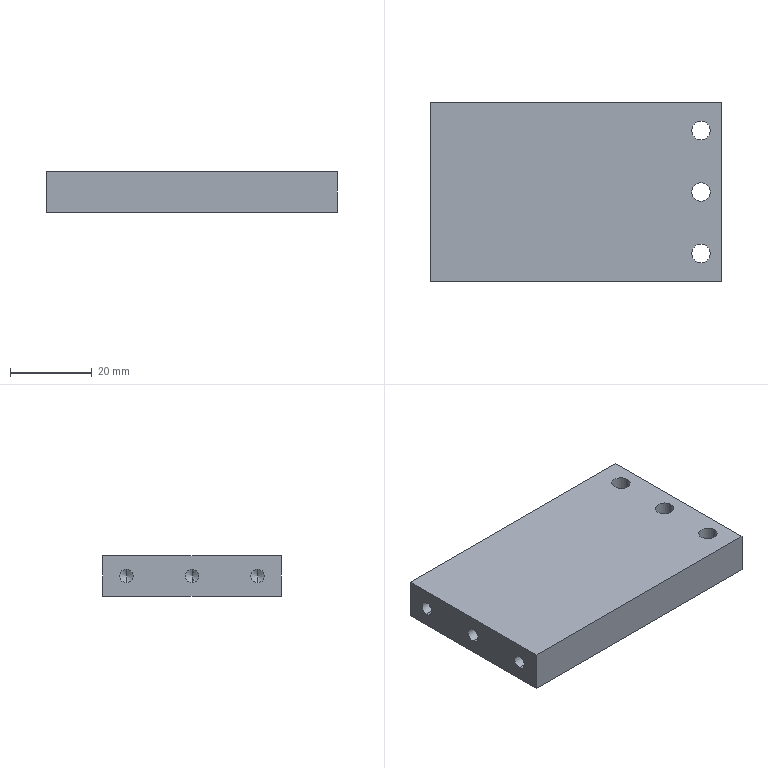Part | SolidWorks | features HoleWzd 2, Extrusion 1 | 1 solid | 33 faces | box 71 x 43.6 x 10 mm | volume 29737 mm3 | cylinder 18 | plane 9 | cone 6 | commonest cylinder face diameters 3.3 x6 4.5 x6 8 x6
STEP:
#1=CARTESIAN_POINT('',(10.1,37.8,-6.65));
#2=VERTEX_POINT('',#1);
#3=CARTESIAN_POINT('',(10.1,37.8,-3.35));
#4=VERTEX_POINT('',#3);
#5=CARTESIAN_POINT('',(10.1,37.8,-5.));
#6=DIRECTION('',(-1.,0.,0.));
#7=DIRECTION('',(0.,0.,1.));
#8=AXIS2_PLACEMENT_3D('',#5,#6,#7);
#9=CIRCLE('',#8,1.65);
#10=EDGE_CURVE('',#2,#4,#9,.T.);
#11=ORIENTED_EDGE('',*,*,#10,.F.);
#12=CARTESIAN_POINT('',(0.,37.8,-6.65));
#13=VERTEX_POINT('',#12);
#14=CARTESIAN_POINT('',(0.,37.8,-6.65));
#15=DIRECTION('',(-1.,0.,0.));
#16=VECTOR('',#15,1000.);
#17=LINE('',#14,#16);
#18=EDGE_CURVE('',#2,#13,#17,.T.);
#19=ORIENTED_EDGE('',*,*,#18,.T.);
#20=CARTESIAN_POINT('',(0.,37.8,-3.35));
#21=VERTEX_POINT('',#20);
#22=CARTESIAN_POINT('',(0.,37.8,-5.));
#23=DIRECTION('',(-1.,0.,0.));
#24=DIRECTION('',(0.,0.,1.));
#25=AXIS2_PLACEMENT_3D('',#22,#23,#24);
#26=CIRCLE('',#25,1.65);
#27=EDGE_CURVE('',#13,#21,#26,.T.);
#28=ORIENTED_EDGE('',*,*,#27,.T.);
#29=CARTESIAN_POINT('',(0.,37.8,-3.35));
#30=DIRECTION('',(-1.,0.,0.));
#31=VECTOR('',#30,1000.);
#32=LINE('',#29,#31);
#33=EDGE_CURVE('',#4,#21,#32,.T.);
#34=ORIENTED_EDGE('',*,*,#33,.F.);
#35=EDGE_LOOP('',(#11,#19,#28,#34));
#36=FACE_OUTER_BOUND('',#35,.T.);
#37=CARTESIAN_POINT('',(0.,37.8,-5.));
#38=DIRECTION('',(-1.,0.,0.));
#39=DIRECTION('',(0.,0.,1.));
#40=AXIS2_PLACEMENT_3D('',#37,#38,#39);
#41=CYLINDRICAL_SURFACE('',#40,1.65);
#42=ADVANCED_FACE('',(#36),#41,.F.);
#43=CARTESIAN_POINT('',(11.091,37.8,-5.));
#44=VERTEX_POINT('',#43);
#45=CARTESIAN_POINT('',(10.1,37.8,-3.35));
#46=DIRECTION('',(-0.515,0.,0.8572));
#47=VECTOR('',#46,1000.);
#48=LINE('',#45,#47);
#49=EDGE_CURVE('',#44,#4,#48,.T.);
#50=ORIENTED_EDGE('',*,*,#49,.F.);
#51=CARTESIAN_POINT('',(10.1,37.8,-6.65));
#52=DIRECTION('',(-0.515,0.,-0.8572));
#53=VECTOR('',#52,1000.);
#54=LINE('',#51,#53);
#55=EDGE_CURVE('',#44,#2,#54,.T.);
#56=ORIENTED_EDGE('',*,*,#55,.T.);
#57=ORIENTED_EDGE('',*,*,#10,.T.);
#58=EDGE_LOOP('',(#50,#56,#57));
#59=FACE_OUTER_BOUND('',#58,.T.);
#60=CARTESIAN_POINT('',(10.1,37.8,-5.));
#61=DIRECTION('',(-1.,0.,0.));
#62=DIRECTION('',(0.,0.,1.));
#63=AXIS2_PLACEMENT_3D('',#60,#61,#62);
#64=CONICAL_SURFACE('',#63,1.65,1.03);
#65=ADVANCED_FACE('',(#59),#64,.F.);
#66=CARTESIAN_POINT('',(10.1,21.8,-6.65));
#67=VERTEX_POINT('',#66);
#68=CARTESIAN_POINT('',(10.1,21.8,-3.35));
#69=VERTEX_POINT('',#68);
#70=CARTESIAN_POINT('',(10.1,21.8,-5.));
#71=DIRECTION('',(-1.,0.,0.));
#72=DIRECTION('',(0.,0.,1.));
#73=AXIS2_PLACEMENT_3D('',#70,#71,#72);
#74=CIRCLE('',#73,1.65);
#75=EDGE_CURVE('',#67,#69,#74,.T.);
#76=ORIENTED_EDGE('',*,*,#75,.F.);
#77=CARTESIAN_POINT('',(0.,21.8,-6.65));
#78=VERTEX_POINT('',#77);
#79=CARTESIAN_POINT('',(0.,21.8,-6.65));
#80=DIRECTION('',(-1.,0.,0.));
#81=VECTOR('',#80,1000.);
#82=LINE('',#79,#81);
#83=EDGE_CURVE('',#67,#78,#82,.T.);
#84=ORIENTED_EDGE('',*,*,#83,.T.);
#85=CARTESIAN_POINT('',(0.,21.8,-3.35));
#86=VERTEX_POINT('',#85);
#87=CARTESIAN_POINT('',(0.,21.8,-5.));
#88=DIRECTION('',(-1.,0.,0.));
#89=DIRECTION('',(0.,0.,1.));
#90=AXIS2_PLACEMENT_3D('',#87,#88,#89);
#91=CIRCLE('',#90,1.65);
#92=EDGE_CURVE('',#78,#86,#91,.T.);
#93=ORIENTED_EDGE('',*,*,#92,.T.);
#94=CARTESIAN_POINT('',(0.,21.8,-3.35));
#95=DIRECTION('',(-1.,0.,0.));
#96=VECTOR('',#95,1000.);
#97=LINE('',#94,#96);
#98=EDGE_CURVE('',#69,#86,#97,.T.);
#99=ORIENTED_EDGE('',*,*,#98,.F.);
#100=EDGE_LOOP('',(#76,#84,#93,#99));
#101=FACE_OUTER_BOUND('',#100,.T.);
#102=CARTESIAN_POINT('',(0.,21.8,-5.));
#103=DIRECTION('',(-1.,0.,0.));
#104=DIRECTION('',(0.,0.,1.));
#105=AXIS2_PLACEMENT_3D('',#102,#103,#104);
#106=CYLINDRICAL_SURFACE('',#105,1.65);
#107=ADVANCED_FACE('',(#101),#106,.F.);
#108=CARTESIAN_POINT('',(11.091,21.8,-5.));
#109=VERTEX_POINT('',#108);
#110=CARTESIAN_POINT('',(10.1,21.8,-3.35));
#111=DIRECTION('',(-0.515,0.,0.8572));
#112=VECTOR('',#111,1000.);
#113=LINE('',#110,#112);
#114=EDGE_CURVE('',#109,#69,#113,.T.);
#115=ORIENTED_EDGE('',*,*,#114,.F.);
#116=CARTESIAN_POINT('',(10.1,21.8,-6.65));
#117=DIRECTION('',(-0.515,0.,-0.8572));
#118=VECTOR('',#117,1000.);
#119=LINE('',#116,#118);
#120=EDGE_CURVE('',#109,#67,#119,.T.);
#121=ORIENTED_EDGE('',*,*,#120,.T.);
#122=ORIENTED_EDGE('',*,*,#75,.T.);
#123=EDGE_LOOP('',(#115,#121,#122));
#124=FACE_OUTER_BOUND('',#123,.T.);
#125=CARTESIAN_POINT('',(10.1,21.8,-5.));
#126=DIRECTION('',(-1.,0.,0.));
#127=DIRECTION('',(0.,0.,1.));
#128=AXIS2_PLACEMENT_3D('',#125,#126,#127);
#129=CONICAL_SURFACE('',#128,1.65,1.03);
#130=ADVANCED_FACE('',(#124),#129,.F.);
#131=CARTESIAN_POINT('',(10.1,5.8,-6.65));
#132=VERTEX_POINT('',#131);
#133=CARTESIAN_POINT('',(10.1,5.8,-3.35));
#134=VERTEX_POINT('',#133);
#135=CARTESIAN_POINT('',(10.1,5.8,-5.));
#136=DIRECTION('',(-1.,0.,0.));
#137=DIRECTION('',(0.,0.,1.));
#138=AXIS2_PLACEMENT_3D('',#135,#136,#137);
#139=CIRCLE('',#138,1.65);
#140=EDGE_CURVE('',#132,#134,#139,.T.);
#141=ORIENTED_EDGE('',*,*,#140,.F.);
#142=CARTESIAN_POINT('',(0.,5.8,-6.65));
#143=VERTEX_POINT('',#142);
#144=CARTESIAN_POINT('',(0.,5.8,-6.65));
#145=DIRECTION('',(-1.,0.,0.));
#146=VECTOR('',#145,1000.);
#147=LINE('',#144,#146);
#148=EDGE_CURVE('',#132,#143,#147,.T.);
#149=ORIENTED_EDGE('',*,*,#148,.T.);
#150=CARTESIAN_POINT('',(0.,5.8,-3.35));
#151=VERTEX_POINT('',#150);
#152=CARTESIAN_POINT('',(0.,5.8,-5.));
#153=DIRECTION('',(-1.,0.,0.));
#154=DIRECTION('',(0.,0.,1.));
#155=AXIS2_PLACEMENT_3D('',#152,#153,#154);
#156=CIRCLE('',#155,1.65);
#157=EDGE_CURVE('',#143,#151,#156,.T.);
#158=ORIENTED_EDGE('',*,*,#157,.T.);
#159=CARTESIAN_POINT('',(0.,5.8,-3.35));
#160=DIRECTION('',(-1.,0.,0.));
#161=VECTOR('',#160,1000.);
#162=LINE('',#159,#161);
#163=EDGE_CURVE('',#134,#151,#162,.T.);
#164=ORIENTED_EDGE('',*,*,#163,.F.);
#165=EDGE_LOOP('',(#141,#149,#158,#164));
#166=FACE_OUTER_BOUND('',#165,.T.);
#167=CARTESIAN_POINT('',(0.,5.8,-5.));
#168=DIRECTION('',(-1.,0.,0.));
#169=DIRECTION('',(0.,0.,1.));
#170=AXIS2_PLACEMENT_3D('',#167,#168,#169);
#171=CYLINDRICAL_SURFACE('',#170,1.65);
#172=ADVANCED_FACE('',(#166),#171,.F.);
#173=CARTESIAN_POINT('',(11.091,5.8,-5.));
#174=VERTEX_POINT('',#173);
#175=CARTESIAN_POINT('',(10.1,5.8,-3.35));
#176=DIRECTION('',(-0.515,0.,0.8572));
#177=VECTOR('',#176,1000.);
#178=LINE('',#175,#177);
#179=EDGE_CURVE('',#174,#134,#178,.T.);
#180=ORIENTED_EDGE('',*,*,#179,.F.);
#181=CARTESIAN_POINT('',(10.1,5.8,-6.65));
#182=DIRECTION('',(-0.515,0.,-0.8572));
#183=VECTOR('',#182,1000.);
#184=LINE('',#181,#183);
#185=EDGE_CURVE('',#174,#132,#184,.T.);
#186=ORIENTED_EDGE('',*,*,#185,.T.);
#187=ORIENTED_EDGE('',*,*,#140,.T.);
#188=EDGE_LOOP('',(#180,#186,#187));
#189=FACE_OUTER_BOUND('',#188,.T.);
#190=CARTESIAN_POINT('',(10.1,5.8,-5.));
#191=DIRECTION('',(-1.,0.,0.));
#192=DIRECTION('',(0.,0.,1.));
#193=AXIS2_PLACEMENT_3D('',#190,#191,#192);
#194=CONICAL_SURFACE('',#193,1.65,1.03);
#195=ADVANCED_FACE('',(#189),#194,.F.);
#196=CARTESIAN_POINT('',(70.,36.8,-5.4));
#197=VERTEX_POINT('',#196);
#198=CARTESIAN_POINT('',(62.,36.8,-5.4));
#199=VERTEX_POINT('',#198);
#200=CARTESIAN_POINT('',(66.,36.8,-5.4));
#201=DIRECTION('',(0.,0.,-1.));
#202=DIRECTION('',(-1.,0.,0.));
#203=AXIS2_PLACEMENT_3D('',#200,#201,#202);
#204=CIRCLE('',#203,4.);
#205=EDGE_CURVE('',#197,#199,#204,.T.);
#206=ORIENTED_EDGE('',*,*,#205,.F.);
#207=CARTESIAN_POINT('',(70.,36.8,-10.));
#208=VERTEX_POINT('',#207);
#209=CARTESIAN_POINT('',(70.,36.8,-10.));
#210=DIRECTION('',(0.,0.,-1.));
#211=VECTOR('',#210,1000.);
#212=LINE('',#209,#211);
#213=EDGE_CURVE('',#197,#208,#212,.T.);
#214=ORIENTED_EDGE('',*,*,#213,.T.);
#215=CARTESIAN_POINT('',(62.,36.8,-10.));
#216=VERTEX_POINT('',#215);
#217=CARTESIAN_POINT('',(66.,36.8,-10.));
#218=DIRECTION('',(0.,0.,-1.));
#219=DIRECTION('',(-1.,0.,0.));
#220=AXIS2_PLACEMENT_3D('',#217,#218,#219);
#221=CIRCLE('',#220,4.);
#222=EDGE_CURVE('',#208,#216,#221,.T.);
#223=ORIENTED_EDGE('',*,*,#222,.T.);
#224=CARTESIAN_POINT('',(62.,36.8,-10.));
#225=DIRECTION('',(0.,0.,-1.));
#226=VECTOR('',#225,1000.);
#227=LINE('',#224,#226);
#228=EDGE_CURVE('',#199,#216,#227,.T.);
#229=ORIENTED_EDGE('',*,*,#228,.F.);
#230=EDGE_LOOP('',(#206,#214,#223,#229));
#231=FACE_OUTER_BOUND('',#230,.T.);
#232=CARTESIAN_POINT('',(66.,36.8,-10.));
#233=DIRECTION('',(0.,0.,-1.));
#234=DIRECTION('',(-1.,0.,0.));
#235=AXIS2_PLACEMENT_3D('',#232,#233,#234);
#236=CYLINDRICAL_SURFACE('',#235,4.);
#237=ADVANCED_FACE('',(#231),#236,.F.);
#238=CARTESIAN_POINT('',(68.25,36.8,0.));
#239=VERTEX_POINT('',#238);
#240=CARTESIAN_POINT('',(63.75,36.8,0.));
#241=VERTEX_POINT('',#240);
#242=CARTESIAN_POINT('',(66.,36.8,0.));
#243=DIRECTION('',(0.,0.,-1.));
#244=DIRECTION('',(-1.,0.,0.));
#245=AXIS2_PLACEMENT_3D('',#242,#243,#244);
#246=CIRCLE('',#245,2.25);
#247=EDGE_CURVE('',#239,#241,#246,.T.);
#248=ORIENTED_EDGE('',*,*,#247,.F.);
#249=CARTESIAN_POINT('',(68.25,36.8,-5.4));
#250=VERTEX_POINT('',#249);
#251=CARTESIAN_POINT('',(68.25,36.8,-10.));
#252=DIRECTION('',(0.,0.,-1.));
#253=VECTOR('',#252,1000.);
#254=LINE('',#251,#253);
#255=EDGE_CURVE('',#239,#250,#254,.T.);
#256=ORIENTED_EDGE('',*,*,#255,.T.);
#257=CARTESIAN_POINT('',(63.75,36.8,-5.4));
#258=VERTEX_POINT('',#257);
#259=CARTESIAN_POINT('',(66.,36.8,-5.4));
#260=DIRECTION('',(0.,0.,-1.));
#261=DIRECTION('',(-1.,0.,0.));
#262=AXIS2_PLACEMENT_3D('',#259,#260,#261);
#263=CIRCLE('',#262,2.25);
#264=EDGE_CURVE('',#250,#258,#263,.T.);
#265=ORIENTED_EDGE('',*,*,#264,.T.);
#266=CARTESIAN_POINT('',(63.75,36.8,-10.));
#267=DIRECTION('',(0.,0.,-1.));
#268=VECTOR('',#267,1000.);
#269=LINE('',#266,#268);
#270=EDGE_CURVE('',#241,#258,#269,.T.);
#271=ORIENTED_EDGE('',*,*,#270,.F.);
#272=EDGE_LOOP('',(#248,#256,#265,#271));
#273=FACE_OUTER_BOUND('',#272,.T.);
#274=CARTESIAN_POINT('',(66.,36.8,-10.));
#275=DIRECTION('',(0.,0.,-1.));
#276=DIRECTION('',(-1.,0.,0.));
#277=AXIS2_PLACEMENT_3D('',#274,#275,#276);
#278=CYLINDRICAL_SURFACE('',#277,2.25);
#279=ADVANCED_FACE('',(#273),#278,.F.);
#280=CARTESIAN_POINT('',(70.,21.783,-5.4));
#281=VERTEX_POINT('',#280);
#282=CARTESIAN_POINT('',(62.,21.783,-5.4));
#283=VERTEX_POINT('',#282);
#284=CARTESIAN_POINT('',(66.,21.783,-5.4));
#285=DIRECTION('',(0.,0.,-1.));
#286=DIRECTION('',(-1.,0.,0.));
#287=AXIS2_PLACEMENT_3D('',#284,#285,#286);
#288=CIRCLE('',#287,4.);
#289=EDGE_CURVE('',#281,#283,#288,.T.);
#290=ORIENTED_EDGE('',*,*,#289,.F.);
#291=CARTESIAN_POINT('',(70.,21.783,-10.));
#292=VERTEX_POINT('',#291);
#293=CARTESIAN_POINT('',(70.,21.783,-10.));
#294=DIRECTION('',(0.,0.,-1.));
#295=VECTOR('',#294,1000.);
#296=LINE('',#293,#295);
#297=EDGE_CURVE('',#281,#292,#296,.T.);
#298=ORIENTED_EDGE('',*,*,#297,.T.);
#299=CARTESIAN_POINT('',(62.,21.783,-10.));
#300=VERTEX_POINT('',#299);
#301=CARTESIAN_POINT('',(66.,21.783,-10.));
#302=DIRECTION('',(0.,0.,-1.));
#303=DIRECTION('',(-1.,0.,0.));
#304=AXIS2_PLACEMENT_3D('',#301,#302,#303);
#305=CIRCLE('',#304,4.);
#306=EDGE_CURVE('',#292,#300,#305,.T.);
#307=ORIENTED_EDGE('',*,*,#306,.T.);
#308=CARTESIAN_POINT('',(62.,21.783,-10.));
#309=DIRECTION('',(0.,0.,-1.));
#310=VECTOR('',#309,1000.);
#311=LINE('',#308,#310);
#312=EDGE_CURVE('',#283,#300,#311,.T.);
#313=ORIENTED_EDGE('',*,*,#312,.F.);
#314=EDGE_LOOP('',(#290,#298,#307,#313));
#315=FACE_OUTER_BOUND('',#314,.T.);
#316=CARTESIAN_POINT('',(66.,21.783,-10.));
#317=DIRECTION('',(0.,0.,-1.));
#318=DIRECTION('',(-1.,0.,0.));
#319=AXIS2_PLACEMENT_3D('',#316,#317,#318);
#320=CYLINDRICAL_SURFACE('',#319,4.);
#321=ADVANCED_FACE('',(#315),#320,.F.);
#322=CARTESIAN_POINT('',(68.25,21.783,0.));
#323=VERTEX_POINT('',#322);
#324=CARTESIAN_POINT('',(63.75,21.783,0.));
#325=VERTEX_POINT('',#324);
#326=CARTESIAN_POINT('',(66.,21.783,0.));
#327=DIRECTION('',(0.,0.,-1.));
#328=DIRECTION('',(-1.,0.,0.));
#329=AXIS2_PLACEMENT_3D('',#326,#327,#328);
#330=CIRCLE('',#329,2.25);
#331=EDGE_CURVE('',#323,#325,#330,.T.);
#332=ORIENTED_EDGE('',*,*,#331,.F.);
#333=CARTESIAN_POINT('',(68.25,21.783,-5.4));
#334=VERTEX_POINT('',#333);
#335=CARTESIAN_POINT('',(68.25,21.783,-10.));
#336=DIRECTION('',(0.,0.,-1.));
#337=VECTOR('',#336,1000.);
#338=LINE('',#335,#337);
#339=EDGE_CURVE('',#323,#334,#338,.T.);
#340=ORIENTED_EDGE('',*,*,#339,.T.);
#341=CARTESIAN_POINT('',(63.75,21.783,-5.4));
#342=VERTEX_POINT('',#341);
#343=CARTESIAN_POINT('',(66.,21.783,-5.4));
#344=DIRECTION('',(0.,0.,-1.));
#345=DIRECTION('',(-1.,0.,0.));
#346=AXIS2_PLACEMENT_3D('',#343,#344,#345);
#347=CIRCLE('',#346,2.25);
#348=EDGE_CURVE('',#334,#342,#347,.T.);
#349=ORIENTED_EDGE('',*,*,#348,.T.);
#350=CARTESIAN_POINT('',(63.75,21.783,-10.));
#351=DIRECTION('',(0.,0.,-1.));
#352=VECTOR('',#351,1000.);
#353=LINE('',#350,#352);
#354=EDGE_CURVE('',#325,#342,#353,.T.);
#355=ORIENTED_EDGE('',*,*,#354,.F.);
#356=EDGE_LOOP('',(#332,#340,#349,#355));
#357=FACE_OUTER_BOUND('',#356,.T.);
#358=CARTESIAN_POINT('',(66.,21.783,-10.));
#359=DIRECTION('',(0.,0.,-1.));
#360=DIRECTION('',(-1.,0.,0.));
#361=AXIS2_PLACEMENT_3D('',#358,#359,#360);
#362=CYLINDRICAL_SURFACE('',#361,2.25);
#363=ADVANCED_FACE('',(#357),#362,.F.);
#364=CARTESIAN_POINT('',(70.,6.8,-5.4));
#365=VERTEX_POINT('',#364);
#366=CARTESIAN_POINT('',(62.,6.8,-5.4));
#367=VERTEX_POINT('',#366);
#368=CARTESIAN_POINT('',(66.,6.8,-5.4));
#369=DIRECTION('',(0.,0.,-1.));
#370=DIRECTION('',(-1.,0.,0.));
#371=AXIS2_PLACEMENT_3D('',#368,#369,#370);
#372=CIRCLE('',#371,4.);
#373=EDGE_CURVE('',#365,#367,#372,.T.);
#374=ORIENTED_EDGE('',*,*,#373,.F.);
#375=CARTESIAN_POINT('',(70.,6.8,-10.));
#376=VERTEX_POINT('',#375);
#377=CARTESIAN_POINT('',(70.,6.8,-10.));
#378=DIRECTION('',(0.,0.,-1.));
#379=VECTOR('',#378,1000.);
#380=LINE('',#377,#379);
#381=EDGE_CURVE('',#365,#376,#380,.T.);
#382=ORIENTED_EDGE('',*,*,#381,.T.);
#383=CARTESIAN_POINT('',(62.,6.8,-10.));
#384=VERTEX_POINT('',#383);
#385=CARTESIAN_POINT('',(66.,6.8,-10.));
#386=DIRECTION('',(0.,0.,-1.));
#387=DIRECTION('',(-1.,0.,0.));
#388=AXIS2_PLACEMENT_3D('',#385,#386,#387);
#389=CIRCLE('',#388,4.);
#390=EDGE_CURVE('',#376,#384,#389,.T.);
#391=ORIENTED_EDGE('',*,*,#390,.T.);
#392=CARTESIAN_POINT('',(62.,6.8,-10.));
#393=DIRECTION('',(0.,0.,-1.));
#394=VECTOR('',#393,1000.);
#395=LINE('',#392,#394);
#396=EDGE_CURVE('',#367,#384,#395,.T.);
#397=ORIENTED_EDGE('',*,*,#396,.F.);
#398=EDGE_LOOP('',(#374,#382,#391,#397));
#399=FACE_OUTER_BOUND('',#398,.T.);
#400=CARTESIAN_POINT('',(66.,6.8,-10.));
#401=DIRECTION('',(0.,0.,-1.));
#402=DIRECTION('',(-1.,0.,0.));
#403=AXIS2_PLACEMENT_3D('',#400,#401,#402);
#404=CYLINDRICAL_SURFACE('',#403,4.);
#405=ADVANCED_FACE('',(#399),#404,.F.);
#406=CARTESIAN_POINT('',(68.25,6.8,0.));
#407=VERTEX_POINT('',#406);
#408=CARTESIAN_POINT('',(63.75,6.8,0.));
#409=VERTEX_POINT('',#408);
#410=CARTESIAN_POINT('',(66.,6.8,0.));
#411=DIRECTION('',(0.,0.,-1.));
#412=DIRECTION('',(-1.,0.,0.));
#413=AXIS2_PLACEMENT_3D('',#410,#411,#412);
#414=CIRCLE('',#413,2.25);
#415=EDGE_CURVE('',#407,#409,#414,.T.);
#416=ORIENTED_EDGE('',*,*,#415,.F.);
#417=CARTESIAN_POINT('',(68.25,6.8,-5.4));
#418=VERTEX_POINT('',#417);
#419=CARTESIAN_POINT('',(68.25,6.8,-10.));
#420=DIRECTION('',(0.,0.,-1.));
#421=VECTOR('',#420,1000.);
#422=LINE('',#419,#421);
#423=EDGE_CURVE('',#407,#418,#422,.T.);
#424=ORIENTED_EDGE('',*,*,#423,.T.);
#425=CARTESIAN_POINT('',(63.75,6.8,-5.4));
#426=VERTEX_POINT('',#425);
#427=CARTESIAN_POINT('',(66.,6.8,-5.4));
#428=DIRECTION('',(0.,0.,-1.));
#429=DIRECTION('',(-1.,0.,0.));
#430=AXIS2_PLACEMENT_3D('',#427,#428,#429);
#431=CIRCLE('',#430,2.25);
#432=EDGE_CURVE('',#418,#426,#431,.T.);
#433=ORIENTED_EDGE('',*,*,#432,.T.);
#434=CARTESIAN_POINT('',(63.75,6.8,-10.));
#435=DIRECTION('',(0.,0.,-1.));
#436=VECTOR('',#435,1000.);
#437=LINE('',#434,#436);
#438=EDGE_CURVE('',#409,#426,#437,.T.);
#439=ORIENTED_EDGE('',*,*,#438,.F.);
#440=EDGE_LOOP('',(#416,#424,#433,#439));
#441=FACE_OUTER_BOUND('',#440,.T.);
#442=CARTESIAN_POINT('',(66.,6.8,-10.));
#443=DIRECTION('',(0.,0.,-1.));
#444=DIRECTION('',(-1.,0.,0.));
#445=AXIS2_PLACEMENT_3D('',#442,#443,#444);
#446=CYLINDRICAL_SURFACE('',#445,2.25);
#447=ADVANCED_FACE('',(#441),#446,.F.);
#448=CARTESIAN_POINT('',(0.,37.8,-5.));
#449=DIRECTION('',(-1.,0.,0.));
#450=DIRECTION('',(0.,0.,1.));
#451=AXIS2_PLACEMENT_3D('',#448,#449,#450);
#452=CIRCLE('',#451,1.65);
#453=EDGE_CURVE('',#21,#13,#452,.T.);
#454=ORIENTED_EDGE('',*,*,#453,.F.);
#455=ORIENTED_EDGE('',*,*,#27,.F.);
#456=EDGE_LOOP('',(#454,#455));
#457=FACE_BOUND('',#456,.T.);
#458=CARTESIAN_POINT('',(0.,21.8,-5.));
#459=DIRECTION('',(-1.,0.,0.));
#460=DIRECTION('',(0.,0.,1.));
#461=AXIS2_PLACEMENT_3D('',#458,#459,#460);
#462=CIRCLE('',#461,1.65);
#463=EDGE_CURVE('',#86,#78,#462,.T.);
#464=ORIENTED_EDGE('',*,*,#463,.F.);
#465=ORIENTED_EDGE('',*,*,#92,.F.);
#466=EDGE_LOOP('',(#464,#465));
#467=FACE_BOUND('',#466,.T.);
#468=CARTESIAN_POINT('',(0.,5.8,-5.));
#469=DIRECTION('',(-1.,0.,0.));
#470=DIRECTION('',(0.,0.,1.));
#471=AXIS2_PLACEMENT_3D('',#468,#469,#470);
#472=CIRCLE('',#471,1.65);
#473=EDGE_CURVE('',#151,#143,#472,.T.);
#474=ORIENTED_EDGE('',*,*,#473,.F.);
#475=ORIENTED_EDGE('',*,*,#157,.F.);
#476=EDGE_LOOP('',(#474,#475));
#477=FACE_BOUND('',#476,.T.);
#478=CARTESIAN_POINT('',(0.,0.,-10.));
#479=VERTEX_POINT('',#478);
#480=CARTESIAN_POINT('',(0.,0.,0.));
#481=VERTEX_POINT('',#480);
#482=CARTESIAN_POINT('',(0.,0.,0.));
#483=DIRECTION('',(0.,0.,1.));
#484=VECTOR('',#483,1000.);
#485=LINE('',#482,#484);
#486=EDGE_CURVE('',#479,#481,#485,.T.);
#487=ORIENTED_EDGE('',*,*,#486,.T.);
#488=CARTESIAN_POINT('',(0.,43.6,0.));
#489=VERTEX_POINT('',#488);
#490=CARTESIAN_POINT('',(0.,43.6,0.));
#491=DIRECTION('',(0.,-1.,0.));
#492=VECTOR('',#491,1000.);
#493=LINE('',#490,#492);
#494=EDGE_CURVE('',#489,#481,#493,.T.);
#495=ORIENTED_EDGE('',*,*,#494,.F.);
#496=CARTESIAN_POINT('',(0.,43.6,-10.));
#497=VERTEX_POINT('',#496);
#498=CARTESIAN_POINT('',(0.,43.6,0.));
#499=DIRECTION('',(0.,0.,1.));
#500=VECTOR('',#499,1000.);
#501=LINE('',#498,#500);
#502=EDGE_CURVE('',#497,#489,#501,.T.);
#503=ORIENTED_EDGE('',*,*,#502,.F.);
#504=CARTESIAN_POINT('',(0.,43.6,-10.));
#505=DIRECTION('',(0.,-1.,0.));
#506=VECTOR('',#505,1000.);
#507=LINE('',#504,#506);
#508=EDGE_CURVE('',#497,#479,#507,.T.);
#509=ORIENTED_EDGE('',*,*,#508,.T.);
#510=EDGE_LOOP('',(#487,#495,#503,#509));
#511=FACE_OUTER_BOUND('',#510,.T.);
#512=CARTESIAN_POINT('',(0.,43.6,0.));
#513=DIRECTION('',(1.,0.,0.));
#514=DIRECTION('',(0.,0.,-1.));
#515=AXIS2_PLACEMENT_3D('',#512,#513,#514);
#516=PLANE('',#515);
#517=ADVANCED_FACE('',(#457,#467,#477,#511),#516,.F.);
#518=CARTESIAN_POINT('',(66.,36.8,0.));
#519=DIRECTION('',(0.,0.,-1.));
#520=DIRECTION('',(-1.,0.,0.));
#521=AXIS2_PLACEMENT_3D('',#518,#519,#520);
#522=CIRCLE('',#521,2.25);
#523=EDGE_CURVE('',#241,#239,#522,.T.);
#524=ORIENTED_EDGE('',*,*,#523,.T.);
#525=ORIENTED_EDGE('',*,*,#247,.T.);
#526=EDGE_LOOP('',(#524,#525));
#527=FACE_BOUND('',#526,.T.);
#528=CARTESIAN_POINT('',(66.,21.783,0.));
#529=DIRECTION('',(0.,0.,-1.));
#530=DIRECTION('',(-1.,0.,0.));
#531=AXIS2_PLACEMENT_3D('',#528,#529,#530);
#532=CIRCLE('',#531,2.25);
#533=EDGE_CURVE('',#325,#323,#532,.T.);
#534=ORIENTED_EDGE('',*,*,#533,.T.);
#535=ORIENTED_EDGE('',*,*,#331,.T.);
#536=EDGE_LOOP('',(#534,#535));
#537=FACE_BOUND('',#536,.T.);
#538=CARTESIAN_POINT('',(66.,6.8,0.));
#539=DIRECTION('',(0.,0.,-1.));
#540=DIRECTION('',(-1.,0.,0.));
#541=AXIS2_PLACEMENT_3D('',#538,#539,#540);
#542=CIRCLE('',#541,2.25);
#543=EDGE_CURVE('',#409,#407,#542,.T.);
#544=ORIENTED_EDGE('',*,*,#543,.T.);
#545=ORIENTED_EDGE('',*,*,#415,.T.);
#546=EDGE_LOOP('',(#544,#545));
#547=FACE_BOUND('',#546,.T.);
#548=CARTESIAN_POINT('',(71.,0.,0.));
#549=VERTEX_POINT('',#548);
#550=CARTESIAN_POINT('',(0.,0.,0.));
#551=DIRECTION('',(1.,0.,0.));
#552=VECTOR('',#551,1000.);
#553=LINE('',#550,#552);
#554=EDGE_CURVE('',#481,#549,#553,.T.);
#555=ORIENTED_EDGE('',*,*,#554,.T.);
#556=CARTESIAN_POINT('',(71.,43.6,0.));
#557=VERTEX_POINT('',#556);
#558=CARTESIAN_POINT('',(71.,43.6,0.));
#559=DIRECTION('',(0.,-1.,0.));
#560=VECTOR('',#559,1000.);
#561=LINE('',#558,#560);
#562=EDGE_CURVE('',#557,#549,#561,.T.);
#563=ORIENTED_EDGE('',*,*,#562,.F.);
#564=CARTESIAN_POINT('',(0.,43.6,0.));
#565=DIRECTION('',(1.,0.,0.));
#566=VECTOR('',#565,1000.);
#567=LINE('',#564,#566);
#568=EDGE_CURVE('',#489,#557,#567,.T.);
#569=ORIENTED_EDGE('',*,*,#568,.F.);
#570=ORIENTED_EDGE('',*,*,#494,.T.);
#571=EDGE_LOOP('',(#555,#563,#569,#570));
#572=FACE_OUTER_BOUND('',#571,.T.);
#573=CARTESIAN_POINT('',(0.,43.6,0.));
#574=DIRECTION('',(0.,0.,-1.));
#575=DIRECTION('',(-1.,0.,0.));
#576=AXIS2_PLACEMENT_3D('',#573,#574,#575);
#577=PLANE('',#576);
#578=ADVANCED_FACE('',(#527,#537,#547,#572),#577,.F.);
#579=CARTESIAN_POINT('',(71.,0.,-10.));
#580=VERTEX_POINT('',#579);
#581=CARTESIAN_POINT('',(71.,0.,0.));
#582=DIRECTION('',(0.,0.,-1.));
#583=VECTOR('',#582,1000.);
#584=LINE('',#581,#583);
#585=EDGE_CURVE('',#549,#580,#584,.T.);
#586=ORIENTED_EDGE('',*,*,#585,.T.);
#587=CARTESIAN_POINT('',(71.,43.6,-10.));
#588=VERTEX_POINT('',#587);
#589=CARTESIAN_POINT('',(71.,43.6,-10.));
#590=DIRECTION('',(0.,-1.,0.));
#591=VECTOR('',#590,1000.);
#592=LINE('',#589,#591);
#593=EDGE_CURVE('',#588,#580,#592,.T.);
#594=ORIENTED_EDGE('',*,*,#593,.F.);
#595=CARTESIAN_POINT('',(71.,43.6,0.));
#596=DIRECTION('',(0.,0.,-1.));
#597=VECTOR('',#596,1000.);
#598=LINE('',#595,#597);
#599=EDGE_CURVE('',#557,#588,#598,.T.);
#600=ORIENTED_EDGE('',*,*,#599,.F.);
#601=ORIENTED_EDGE('',*,*,#562,.T.);
#602=EDGE_LOOP('',(#586,#594,#600,#601));
#603=FACE_OUTER_BOUND('',#602,.T.);
#604=CARTESIAN_POINT('',(71.,43.6,0.));
#605=DIRECTION('',(-1.,0.,0.));
#606=DIRECTION('',(0.,0.,1.));
#607=AXIS2_PLACEMENT_3D('',#604,#605,#606);
#608=PLANE('',#607);
#609=ADVANCED_FACE('',(#603),#608,.F.);
#610=CARTESIAN_POINT('',(66.,36.8,-10.));
#611=DIRECTION('',(0.,0.,-1.));
#612=DIRECTION('',(-1.,0.,0.));
#613=AXIS2_PLACEMENT_3D('',#610,#611,#612);
#614=CIRCLE('',#613,4.);
#615=EDGE_CURVE('',#216,#208,#614,.T.);
#616=ORIENTED_EDGE('',*,*,#615,.F.);
#617=ORIENTED_EDGE('',*,*,#222,.F.);
#618=EDGE_LOOP('',(#616,#617));
#619=FACE_BOUND('',#618,.T.);
#620=CARTESIAN_POINT('',(66.,21.783,-10.));
#621=DIRECTION('',(0.,0.,-1.));
#622=DIRECTION('',(-1.,0.,0.));
#623=AXIS2_PLACEMENT_3D('',#620,#621,#622);
#624=CIRCLE('',#623,4.);
#625=EDGE_CURVE('',#300,#292,#624,.T.);
#626=ORIENTED_EDGE('',*,*,#625,.F.);
#627=ORIENTED_EDGE('',*,*,#306,.F.);
#628=EDGE_LOOP('',(#626,#627));
#629=FACE_BOUND('',#628,.T.);
#630=CARTESIAN_POINT('',(66.,6.8,-10.));
#631=DIRECTION('',(0.,0.,-1.));
#632=DIRECTION('',(-1.,0.,0.));
#633=AXIS2_PLACEMENT_3D('',#630,#631,#632);
#634=CIRCLE('',#633,4.);
#635=EDGE_CURVE('',#384,#376,#634,.T.);
#636=ORIENTED_EDGE('',*,*,#635,.F.);
#637=ORIENTED_EDGE('',*,*,#390,.F.);
#638=EDGE_LOOP('',(#636,#637));
#639=FACE_BOUND('',#638,.T.);
#640=CARTESIAN_POINT('',(0.,0.,-10.));
#641=DIRECTION('',(-1.,0.,0.));
#642=VECTOR('',#641,1000.);
#643=LINE('',#640,#642);
#644=EDGE_CURVE('',#580,#479,#643,.T.);
#645=ORIENTED_EDGE('',*,*,#644,.T.);
#646=ORIENTED_EDGE('',*,*,#508,.F.);
#647=CARTESIAN_POINT('',(0.,43.6,-10.));
#648=DIRECTION('',(-1.,0.,0.));
#649=VECTOR('',#648,1000.);
#650=LINE('',#647,#649);
#651=EDGE_CURVE('',#588,#497,#650,.T.);
#652=ORIENTED_EDGE('',*,*,#651,.F.);
#653=ORIENTED_EDGE('',*,*,#593,.T.);
#654=EDGE_LOOP('',(#645,#646,#652,#653));
#655=FACE_OUTER_BOUND('',#654,.T.);
#656=CARTESIAN_POINT('',(0.,43.6,-10.));
#657=DIRECTION('',(0.,0.,1.));
#658=DIRECTION('',(1.,0.,0.));
#659=AXIS2_PLACEMENT_3D('',#656,#657,#658);
#660=PLANE('',#659);
#661=ADVANCED_FACE('',(#619,#629,#639,#655),#660,.F.);
#662=ORIENTED_EDGE('',*,*,#502,.T.);
#663=ORIENTED_EDGE('',*,*,#568,.T.);
#664=ORIENTED_EDGE('',*,*,#599,.T.);
#665=ORIENTED_EDGE('',*,*,#651,.T.);
#666=EDGE_LOOP('',(#662,#663,#664,#665));
#667=FACE_OUTER_BOUND('',#666,.T.);
#668=CARTESIAN_POINT('',(0.,43.6,0.));
#669=DIRECTION('',(0.,-1.,0.));
#670=DIRECTION('',(0.,0.,-1.));
#671=AXIS2_PLACEMENT_3D('',#668,#669,#670);
#672=PLANE('',#671);
#673=ADVANCED_FACE('',(#667),#672,.F.);
#674=ORIENTED_EDGE('',*,*,#486,.F.);
#675=ORIENTED_EDGE('',*,*,#644,.F.);
#676=ORIENTED_EDGE('',*,*,#585,.F.);
#677=ORIENTED_EDGE('',*,*,#554,.F.);
#678=EDGE_LOOP('',(#674,#675,#676,#677));
#679=FACE_OUTER_BOUND('',#678,.T.);
#680=CARTESIAN_POINT('',(0.,0.,0.));
#681=DIRECTION('',(0.,-1.,0.));
#682=DIRECTION('',(0.,0.,-1.));
#683=AXIS2_PLACEMENT_3D('',#680,#681,#682);
#684=PLANE('',#683);
#685=ADVANCED_FACE('',(#679),#684,.T.);
#686=ORIENTED_EDGE('',*,*,#423,.F.);
#687=ORIENTED_EDGE('',*,*,#543,.F.);
#688=ORIENTED_EDGE('',*,*,#438,.T.);
#689=CARTESIAN_POINT('',(66.,6.8,-5.4));
#690=DIRECTION('',(0.,0.,-1.));
#691=DIRECTION('',(-1.,0.,0.));
#692=AXIS2_PLACEMENT_3D('',#689,#690,#691);
#693=CIRCLE('',#692,2.25);
#694=EDGE_CURVE('',#426,#418,#693,.T.);
#695=ORIENTED_EDGE('',*,*,#694,.T.);
#696=EDGE_LOOP('',(#686,#687,#688,#695));
#697=FACE_OUTER_BOUND('',#696,.T.);
#698=CARTESIAN_POINT('',(66.,6.8,-10.));
#699=DIRECTION('',(0.,0.,-1.));
#700=DIRECTION('',(-1.,0.,0.));
#701=AXIS2_PLACEMENT_3D('',#698,#699,#700);
#702=CYLINDRICAL_SURFACE('',#701,2.25);
#703=ADVANCED_FACE('',(#697),#702,.F.);
#704=ORIENTED_EDGE('',*,*,#694,.F.);
#705=ORIENTED_EDGE('',*,*,#432,.F.);
#706=EDGE_LOOP('',(#704,#705));
#707=FACE_BOUND('',#706,.T.);
#708=CARTESIAN_POINT('',(66.,6.8,-5.4));
#709=DIRECTION('',(0.,0.,-1.));
#710=DIRECTION('',(-1.,0.,0.));
#711=AXIS2_PLACEMENT_3D('',#708,#709,#710);
#712=CIRCLE('',#711,4.);
#713=EDGE_CURVE('',#367,#365,#712,.T.);
#714=ORIENTED_EDGE('',*,*,#713,.T.);
#715=ORIENTED_EDGE('',*,*,#373,.T.);
#716=EDGE_LOOP('',(#714,#715));
#717=FACE_OUTER_BOUND('',#716,.T.);
#718=CARTESIAN_POINT('',(68.25,6.8,-5.4));
#719=DIRECTION('',(0.,0.,1.));
#720=DIRECTION('',(1.,0.,0.));
#721=AXIS2_PLACEMENT_3D('',#718,#719,#720);
#722=PLANE('',#721);
#723=ADVANCED_FACE('',(#707,#717),#722,.F.);
#724=ORIENTED_EDGE('',*,*,#381,.F.);
#725=ORIENTED_EDGE('',*,*,#713,.F.);
#726=ORIENTED_EDGE('',*,*,#396,.T.);
#727=ORIENTED_EDGE('',*,*,#635,.T.);
#728=EDGE_LOOP('',(#724,#725,#726,#727));
#729=FACE_OUTER_BOUND('',#728,.T.);
#730=CARTESIAN_POINT('',(66.,6.8,-10.));
#731=DIRECTION('',(0.,0.,-1.));
#732=DIRECTION('',(-1.,0.,0.));
#733=AXIS2_PLACEMENT_3D('',#730,#731,#732);
#734=CYLINDRICAL_SURFACE('',#733,4.);
#735=ADVANCED_FACE('',(#729),#734,.F.);
#736=ORIENTED_EDGE('',*,*,#339,.F.);
#737=ORIENTED_EDGE('',*,*,#533,.F.);
#738=ORIENTED_EDGE('',*,*,#354,.T.);
#739=CARTESIAN_POINT('',(66.,21.783,-5.4));
#740=DIRECTION('',(0.,0.,-1.));
#741=DIRECTION('',(-1.,0.,0.));
#742=AXIS2_PLACEMENT_3D('',#739,#740,#741);
#743=CIRCLE('',#742,2.25);
#744=EDGE_CURVE('',#342,#334,#743,.T.);
#745=ORIENTED_EDGE('',*,*,#744,.T.);
#746=EDGE_LOOP('',(#736,#737,#738,#745));
#747=FACE_OUTER_BOUND('',#746,.T.);
#748=CARTESIAN_POINT('',(66.,21.783,-10.));
#749=DIRECTION('',(0.,0.,-1.));
#750=DIRECTION('',(-1.,0.,0.));
#751=AXIS2_PLACEMENT_3D('',#748,#749,#750);
#752=CYLINDRICAL_SURFACE('',#751,2.25);
#753=ADVANCED_FACE('',(#747),#752,.F.);
#754=ORIENTED_EDGE('',*,*,#744,.F.);
#755=ORIENTED_EDGE('',*,*,#348,.F.);
#756=EDGE_LOOP('',(#754,#755));
#757=FACE_BOUND('',#756,.T.);
#758=CARTESIAN_POINT('',(66.,21.783,-5.4));
#759=DIRECTION('',(0.,0.,-1.));
#760=DIRECTION('',(-1.,0.,0.));
#761=AXIS2_PLACEMENT_3D('',#758,#759,#760);
#762=CIRCLE('',#761,4.);
#763=EDGE_CURVE('',#283,#281,#762,.T.);
#764=ORIENTED_EDGE('',*,*,#763,.T.);
#765=ORIENTED_EDGE('',*,*,#289,.T.);
#766=EDGE_LOOP('',(#764,#765));
#767=FACE_OUTER_BOUND('',#766,.T.);
#768=CARTESIAN_POINT('',(68.25,21.783,-5.4));
#769=DIRECTION('',(0.,0.,1.));
#770=DIRECTION('',(1.,0.,0.));
#771=AXIS2_PLACEMENT_3D('',#768,#769,#770);
#772=PLANE('',#771);
#773=ADVANCED_FACE('',(#757,#767),#772,.F.);
#774=ORIENTED_EDGE('',*,*,#297,.F.);
#775=ORIENTED_EDGE('',*,*,#763,.F.);
#776=ORIENTED_EDGE('',*,*,#312,.T.);
#777=ORIENTED_EDGE('',*,*,#625,.T.);
#778=EDGE_LOOP('',(#774,#775,#776,#777));
#779=FACE_OUTER_BOUND('',#778,.T.);
#780=CARTESIAN_POINT('',(66.,21.783,-10.));
#781=DIRECTION('',(0.,0.,-1.));
#782=DIRECTION('',(-1.,0.,0.));
#783=AXIS2_PLACEMENT_3D('',#780,#781,#782);
#784=CYLINDRICAL_SURFACE('',#783,4.);
#785=ADVANCED_FACE('',(#779),#784,.F.);
#786=ORIENTED_EDGE('',*,*,#255,.F.);
#787=ORIENTED_EDGE('',*,*,#523,.F.);
#788=ORIENTED_EDGE('',*,*,#270,.T.);
#789=CARTESIAN_POINT('',(66.,36.8,-5.4));
#790=DIRECTION('',(0.,0.,-1.));
#791=DIRECTION('',(-1.,0.,0.));
#792=AXIS2_PLACEMENT_3D('',#789,#790,#791);
#793=CIRCLE('',#792,2.25);
#794=EDGE_CURVE('',#258,#250,#793,.T.);
#795=ORIENTED_EDGE('',*,*,#794,.T.);
#796=EDGE_LOOP('',(#786,#787,#788,#795));
#797=FACE_OUTER_BOUND('',#796,.T.);
#798=CARTESIAN_POINT('',(66.,36.8,-10.));
#799=DIRECTION('',(0.,0.,-1.));
#800=DIRECTION('',(-1.,0.,0.));
#801=AXIS2_PLACEMENT_3D('',#798,#799,#800);
#802=CYLINDRICAL_SURFACE('',#801,2.25);
#803=ADVANCED_FACE('',(#797),#802,.F.);
#804=ORIENTED_EDGE('',*,*,#794,.F.);
#805=ORIENTED_EDGE('',*,*,#264,.F.);
#806=EDGE_LOOP('',(#804,#805));
#807=FACE_BOUND('',#806,.T.);
#808=CARTESIAN_POINT('',(66.,36.8,-5.4));
#809=DIRECTION('',(0.,0.,-1.));
#810=DIRECTION('',(-1.,0.,0.));
#811=AXIS2_PLACEMENT_3D('',#808,#809,#810);
#812=CIRCLE('',#811,4.);
#813=EDGE_CURVE('',#199,#197,#812,.T.);
#814=ORIENTED_EDGE('',*,*,#813,.T.);
#815=ORIENTED_EDGE('',*,*,#205,.T.);
#816=EDGE_LOOP('',(#814,#815));
#817=FACE_OUTER_BOUND('',#816,.T.);
#818=CARTESIAN_POINT('',(68.25,36.8,-5.4));
#819=DIRECTION('',(0.,0.,1.));
#820=DIRECTION('',(1.,0.,0.));
#821=AXIS2_PLACEMENT_3D('',#818,#819,#820);
#822=PLANE('',#821);
#823=ADVANCED_FACE('',(#807,#817),#822,.F.);
#824=ORIENTED_EDGE('',*,*,#213,.F.);
#825=ORIENTED_EDGE('',*,*,#813,.F.);
#826=ORIENTED_EDGE('',*,*,#228,.T.);
#827=ORIENTED_EDGE('',*,*,#615,.T.);
#828=EDGE_LOOP('',(#824,#825,#826,#827));
#829=FACE_OUTER_BOUND('',#828,.T.);
#830=CARTESIAN_POINT('',(66.,36.8,-10.));
#831=DIRECTION('',(0.,0.,-1.));
#832=DIRECTION('',(-1.,0.,0.));
#833=AXIS2_PLACEMENT_3D('',#830,#831,#832);
#834=CYLINDRICAL_SURFACE('',#833,4.);
#835=ADVANCED_FACE('',(#829),#834,.F.);
#836=ORIENTED_EDGE('',*,*,#185,.F.);
#837=ORIENTED_EDGE('',*,*,#179,.T.);
#838=CARTESIAN_POINT('',(10.1,5.8,-5.));
#839=DIRECTION('',(-1.,0.,0.));
#840=DIRECTION('',(0.,0.,1.));
#841=AXIS2_PLACEMENT_3D('',#838,#839,#840);
#842=CIRCLE('',#841,1.65);
#843=EDGE_CURVE('',#134,#132,#842,.T.);
#844=ORIENTED_EDGE('',*,*,#843,.T.);
#845=EDGE_LOOP('',(#836,#837,#844));
#846=FACE_OUTER_BOUND('',#845,.T.);
#847=CARTESIAN_POINT('',(10.1,5.8,-5.));
#848=DIRECTION('',(-1.,0.,0.));
#849=DIRECTION('',(0.,0.,1.));
#850=AXIS2_PLACEMENT_3D('',#847,#848,#849);
#851=CONICAL_SURFACE('',#850,1.65,1.03);
#852=ADVANCED_FACE('',(#846),#851,.F.);
#853=ORIENTED_EDGE('',*,*,#148,.F.);
#854=ORIENTED_EDGE('',*,*,#843,.F.);
#855=ORIENTED_EDGE('',*,*,#163,.T.);
#856=ORIENTED_EDGE('',*,*,#473,.T.);
#857=EDGE_LOOP('',(#853,#854,#855,#856));
#858=FACE_OUTER_BOUND('',#857,.T.);
#859=CARTESIAN_POINT('',(0.,5.8,-5.));
#860=DIRECTION('',(-1.,0.,0.));
#861=DIRECTION('',(0.,0.,1.));
#862=AXIS2_PLACEMENT_3D('',#859,#860,#861);
#863=CYLINDRICAL_SURFACE('',#862,1.65);
#864=ADVANCED_FACE('',(#858),#863,.F.);
#865=ORIENTED_EDGE('',*,*,#120,.F.);
#866=ORIENTED_EDGE('',*,*,#114,.T.);
#867=CARTESIAN_POINT('',(10.1,21.8,-5.));
#868=DIRECTION('',(-1.,0.,0.));
#869=DIRECTION('',(0.,0.,1.));
#870=AXIS2_PLACEMENT_3D('',#867,#868,#869);
#871=CIRCLE('',#870,1.65);
#872=EDGE_CURVE('',#69,#67,#871,.T.);
#873=ORIENTED_EDGE('',*,*,#872,.T.);
#874=EDGE_LOOP('',(#865,#866,#873));
#875=FACE_OUTER_BOUND('',#874,.T.);
#876=CARTESIAN_POINT('',(10.1,21.8,-5.));
#877=DIRECTION('',(-1.,0.,0.));
#878=DIRECTION('',(0.,0.,1.));
#879=AXIS2_PLACEMENT_3D('',#876,#877,#878);
#880=CONICAL_SURFACE('',#879,1.65,1.03);
#881=ADVANCED_FACE('',(#875),#880,.F.);
#882=ORIENTED_EDGE('',*,*,#83,.F.);
#883=ORIENTED_EDGE('',*,*,#872,.F.);
#884=ORIENTED_EDGE('',*,*,#98,.T.);
#885=ORIENTED_EDGE('',*,*,#463,.T.);
#886=EDGE_LOOP('',(#882,#883,#884,#885));
#887=FACE_OUTER_BOUND('',#886,.T.);
#888=CARTESIAN_POINT('',(0.,21.8,-5.));
#889=DIRECTION('',(-1.,0.,0.));
#890=DIRECTION('',(0.,0.,1.));
#891=AXIS2_PLACEMENT_3D('',#888,#889,#890);
#892=CYLINDRICAL_SURFACE('',#891,1.65);
#893=ADVANCED_FACE('',(#887),#892,.F.);
#894=ORIENTED_EDGE('',*,*,#55,.F.);
#895=ORIENTED_EDGE('',*,*,#49,.T.);
#896=CARTESIAN_POINT('',(10.1,37.8,-5.));
#897=DIRECTION('',(-1.,0.,0.));
#898=DIRECTION('',(0.,0.,1.));
#899=AXIS2_PLACEMENT_3D('',#896,#897,#898);
#900=CIRCLE('',#899,1.65);
#901=EDGE_CURVE('',#4,#2,#900,.T.);
#902=ORIENTED_EDGE('',*,*,#901,.T.);
#903=EDGE_LOOP('',(#894,#895,#902));
#904=FACE_OUTER_BOUND('',#903,.T.);
#905=CARTESIAN_POINT('',(10.1,37.8,-5.));
#906=DIRECTION('',(-1.,0.,0.));
#907=DIRECTION('',(0.,0.,1.));
#908=AXIS2_PLACEMENT_3D('',#905,#906,#907);
#909=CONICAL_SURFACE('',#908,1.65,1.03);
#910=ADVANCED_FACE('',(#904),#909,.F.);
#911=ORIENTED_EDGE('',*,*,#18,.F.);
#912=ORIENTED_EDGE('',*,*,#901,.F.);
#913=ORIENTED_EDGE('',*,*,#33,.T.);
#914=ORIENTED_EDGE('',*,*,#453,.T.);
#915=EDGE_LOOP('',(#911,#912,#913,#914));
#916=FACE_OUTER_BOUND('',#915,.T.);
#917=CARTESIAN_POINT('',(0.,37.8,-5.));
#918=DIRECTION('',(-1.,0.,0.));
#919=DIRECTION('',(0.,0.,1.));
#920=AXIS2_PLACEMENT_3D('',#917,#918,#919);
#921=CYLINDRICAL_SURFACE('',#920,1.65);
#922=ADVANCED_FACE('',(#916),#921,.F.);
#923=CLOSED_SHELL('',(#42,#65,#107,#130,#172,#195,#237,#279,#321,#363,#405,#447,#517,#578,#609,#661,#673,#685,#703,#723,#735,#753,#773,#785,#803,#823,#835,#852,#864,#881,#893,#910,#922));
#924=MANIFOLD_SOLID_BREP('',#923);
#925=CARTESIAN_POINT('',(0.,0.,0.));
#926=DIRECTION('',(0.,0.,1.));
#927=DIRECTION('',(1.,0.,0.));
#928=AXIS2_PLACEMENT_3D('',#925,#926,#927);
#929=(LENGTH_UNIT()NAMED_UNIT(*)SI_UNIT(.MILLI.,.METRE.));
#930=UNCERTAINTY_MEASURE_WITH_UNIT(LENGTH_MEASURE(0.00001),#929,'','');
#931=(NAMED_UNIT(*)PLANE_ANGLE_UNIT()SI_UNIT($,.RADIAN.));
#932=(NAMED_UNIT(*)SI_UNIT($,.STERADIAN.)SOLID_ANGLE_UNIT());
#933=(GEOMETRIC_REPRESENTATION_CONTEXT(3)GLOBAL_UNCERTAINTY_ASSIGNED_CONTEXT((#930))GLOBAL_UNIT_ASSIGNED_CONTEXT((#929,#931,#932))REPRESENTATION_CONTEXT('',''));
#934=ADVANCED_BREP_SHAPE_REPRESENTATION('',(#924,#928),#933);